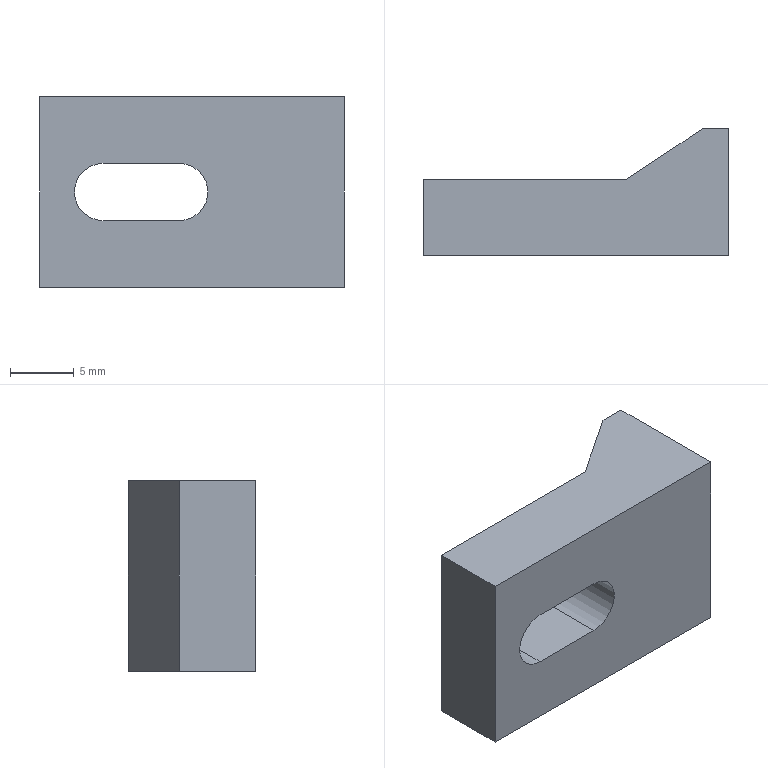Part | SolidWorks | features Extrusion 1, ICE 1 | 1 solid | 12 faces | box 24 x 10 x 15 mm | volume 2203 mm3 | plane 10 | cylinder 2 | commonest cylinder face diameters 4.5 x2
STEP:
#1=CARTESIAN_POINT('',(4.,1.,-7.5));
#2=VERTEX_POINT('',#1);
#3=CARTESIAN_POINT('',(10.,5.,-7.5));
#4=VERTEX_POINT('',#3);
#5=CARTESIAN_POINT('',(0.7692,-1.154,-7.5));
#6=DIRECTION('',(0.8321,0.5547,0.));
#7=VECTOR('',#6,1000.);
#8=LINE('',#5,#7);
#9=EDGE_CURVE('',#2,#4,#8,.T.);
#10=ORIENTED_EDGE('',*,*,#9,.F.);
#11=CARTESIAN_POINT('',(4.,1.,7.5));
#12=VERTEX_POINT('',#11);
#13=CARTESIAN_POINT('',(4.,1.,7.5));
#14=DIRECTION('',(0.,0.,-1.));
#15=VECTOR('',#14,1000.);
#16=LINE('',#13,#15);
#17=EDGE_CURVE('',#12,#2,#16,.T.);
#18=ORIENTED_EDGE('',*,*,#17,.F.);
#19=CARTESIAN_POINT('',(10.,5.,7.5));
#20=VERTEX_POINT('',#19);
#21=CARTESIAN_POINT('',(0.7692,-1.154,7.5));
#22=DIRECTION('',(0.8321,0.5547,0.));
#23=VECTOR('',#22,1000.);
#24=LINE('',#21,#23);
#25=EDGE_CURVE('',#12,#20,#24,.T.);
#26=ORIENTED_EDGE('',*,*,#25,.T.);
#27=CARTESIAN_POINT('',(10.,5.,7.5));
#28=DIRECTION('',(0.,0.,-1.));
#29=VECTOR('',#28,1000.);
#30=LINE('',#27,#29);
#31=EDGE_CURVE('',#20,#4,#30,.T.);
#32=ORIENTED_EDGE('',*,*,#31,.T.);
#33=EDGE_LOOP('',(#10,#18,#26,#32));
#34=FACE_OUTER_BOUND('',#33,.T.);
#35=CARTESIAN_POINT('',(0.7692,-1.154,7.5));
#36=DIRECTION('',(-0.5547,0.8321,0.));
#37=DIRECTION('',(-0.8321,-0.5547,0.));
#38=AXIS2_PLACEMENT_3D('',#35,#36,#37);
#39=PLANE('',#38);
#40=ADVANCED_FACE('',(#34),#39,.T.);
#41=CARTESIAN_POINT('',(-7.,1.,-2.25));
#42=VERTEX_POINT('',#41);
#43=CARTESIAN_POINT('',(-7.,1.,2.25));
#44=VERTEX_POINT('',#43);
#45=CARTESIAN_POINT('',(-7.,1.,0.));
#46=DIRECTION('',(0.,1.,0.));
#47=DIRECTION('',(0.,0.,1.));
#48=AXIS2_PLACEMENT_3D('',#45,#46,#47);
#49=CIRCLE('',#48,2.25);
#50=EDGE_CURVE('',#42,#44,#49,.T.);
#51=ORIENTED_EDGE('',*,*,#50,.F.);
#52=CARTESIAN_POINT('',(-1.,1.,-2.25));
#53=VERTEX_POINT('',#52);
#54=CARTESIAN_POINT('',(-7.,1.,-2.25));
#55=DIRECTION('',(-1.,0.,0.));
#56=VECTOR('',#55,1000.);
#57=LINE('',#54,#56);
#58=EDGE_CURVE('',#53,#42,#57,.T.);
#59=ORIENTED_EDGE('',*,*,#58,.F.);
#60=CARTESIAN_POINT('',(-1.,1.,2.25));
#61=VERTEX_POINT('',#60);
#62=CARTESIAN_POINT('',(-1.,1.,0.));
#63=DIRECTION('',(0.,1.,0.));
#64=DIRECTION('',(0.,0.,1.));
#65=AXIS2_PLACEMENT_3D('',#62,#63,#64);
#66=CIRCLE('',#65,2.25);
#67=EDGE_CURVE('',#61,#53,#66,.T.);
#68=ORIENTED_EDGE('',*,*,#67,.F.);
#69=CARTESIAN_POINT('',(-7.,1.,2.25));
#70=DIRECTION('',(1.,0.,0.));
#71=VECTOR('',#70,1000.);
#72=LINE('',#69,#71);
#73=EDGE_CURVE('',#44,#61,#72,.T.);
#74=ORIENTED_EDGE('',*,*,#73,.F.);
#75=EDGE_LOOP('',(#51,#59,#68,#74));
#76=FACE_BOUND('',#75,.T.);
#77=CARTESIAN_POINT('',(-12.,1.,-7.5));
#78=VERTEX_POINT('',#77);
#79=CARTESIAN_POINT('',(0.,1.,-7.5));
#80=DIRECTION('',(1.,0.,0.));
#81=VECTOR('',#80,1000.);
#82=LINE('',#79,#81);
#83=EDGE_CURVE('',#78,#2,#82,.T.);
#84=ORIENTED_EDGE('',*,*,#83,.F.);
#85=CARTESIAN_POINT('',(-12.,1.,7.5));
#86=VERTEX_POINT('',#85);
#87=CARTESIAN_POINT('',(-12.,1.,7.5));
#88=DIRECTION('',(0.,0.,-1.));
#89=VECTOR('',#88,1000.);
#90=LINE('',#87,#89);
#91=EDGE_CURVE('',#86,#78,#90,.T.);
#92=ORIENTED_EDGE('',*,*,#91,.F.);
#93=CARTESIAN_POINT('',(0.,1.,7.5));
#94=DIRECTION('',(1.,0.,0.));
#95=VECTOR('',#94,1000.);
#96=LINE('',#93,#95);
#97=EDGE_CURVE('',#86,#12,#96,.T.);
#98=ORIENTED_EDGE('',*,*,#97,.T.);
#99=ORIENTED_EDGE('',*,*,#17,.T.);
#100=EDGE_LOOP('',(#84,#92,#98,#99));
#101=FACE_OUTER_BOUND('',#100,.T.);
#102=CARTESIAN_POINT('',(0.,1.,7.5));
#103=DIRECTION('',(0.,1.,0.));
#104=DIRECTION('',(-1.,0.,0.));
#105=AXIS2_PLACEMENT_3D('',#102,#103,#104);
#106=PLANE('',#105);
#107=ADVANCED_FACE('',(#76,#101),#106,.T.);
#108=CARTESIAN_POINT('',(-12.,-5.,-7.5));
#109=VERTEX_POINT('',#108);
#110=CARTESIAN_POINT('',(-12.,0.,-7.5));
#111=DIRECTION('',(0.,1.,0.));
#112=VECTOR('',#111,1000.);
#113=LINE('',#110,#112);
#114=EDGE_CURVE('',#109,#78,#113,.T.);
#115=ORIENTED_EDGE('',*,*,#114,.F.);
#116=CARTESIAN_POINT('',(-12.,-5.,7.5));
#117=VERTEX_POINT('',#116);
#118=CARTESIAN_POINT('',(-12.,-5.,7.5));
#119=DIRECTION('',(0.,0.,-1.));
#120=VECTOR('',#119,1000.);
#121=LINE('',#118,#120);
#122=EDGE_CURVE('',#117,#109,#121,.T.);
#123=ORIENTED_EDGE('',*,*,#122,.F.);
#124=CARTESIAN_POINT('',(-12.,0.,7.5));
#125=DIRECTION('',(0.,1.,0.));
#126=VECTOR('',#125,1000.);
#127=LINE('',#124,#126);
#128=EDGE_CURVE('',#117,#86,#127,.T.);
#129=ORIENTED_EDGE('',*,*,#128,.T.);
#130=ORIENTED_EDGE('',*,*,#91,.T.);
#131=EDGE_LOOP('',(#115,#123,#129,#130));
#132=FACE_OUTER_BOUND('',#131,.T.);
#133=CARTESIAN_POINT('',(-12.,0.,7.5));
#134=DIRECTION('',(-1.,0.,0.));
#135=DIRECTION('',(0.,0.,1.));
#136=AXIS2_PLACEMENT_3D('',#133,#134,#135);
#137=PLANE('',#136);
#138=ADVANCED_FACE('',(#132),#137,.T.);
#139=CARTESIAN_POINT('',(-7.,-5.,-2.25));
#140=VERTEX_POINT('',#139);
#141=CARTESIAN_POINT('',(-1.,-5.,-2.25));
#142=VERTEX_POINT('',#141);
#143=CARTESIAN_POINT('',(-7.,-5.,-2.25));
#144=DIRECTION('',(1.,0.,0.));
#145=VECTOR('',#144,1000.);
#146=LINE('',#143,#145);
#147=EDGE_CURVE('',#140,#142,#146,.T.);
#148=ORIENTED_EDGE('',*,*,#147,.F.);
#149=CARTESIAN_POINT('',(-7.,-5.,2.25));
#150=VERTEX_POINT('',#149);
#151=CARTESIAN_POINT('',(-7.,-5.,0.));
#152=DIRECTION('',(0.,-1.,0.));
#153=DIRECTION('',(0.,0.,1.));
#154=AXIS2_PLACEMENT_3D('',#151,#152,#153);
#155=CIRCLE('',#154,2.25);
#156=EDGE_CURVE('',#150,#140,#155,.T.);
#157=ORIENTED_EDGE('',*,*,#156,.F.);
#158=CARTESIAN_POINT('',(-1.,-5.,2.25));
#159=VERTEX_POINT('',#158);
#160=CARTESIAN_POINT('',(-7.,-5.,2.25));
#161=DIRECTION('',(-1.,0.,0.));
#162=VECTOR('',#161,1000.);
#163=LINE('',#160,#162);
#164=EDGE_CURVE('',#159,#150,#163,.T.);
#165=ORIENTED_EDGE('',*,*,#164,.F.);
#166=CARTESIAN_POINT('',(-1.,-5.,0.));
#167=DIRECTION('',(0.,-1.,0.));
#168=DIRECTION('',(0.,0.,1.));
#169=AXIS2_PLACEMENT_3D('',#166,#167,#168);
#170=CIRCLE('',#169,2.25);
#171=EDGE_CURVE('',#142,#159,#170,.T.);
#172=ORIENTED_EDGE('',*,*,#171,.F.);
#173=EDGE_LOOP('',(#148,#157,#165,#172));
#174=FACE_BOUND('',#173,.T.);
#175=CARTESIAN_POINT('',(12.,-5.,-7.5));
#176=VERTEX_POINT('',#175);
#177=CARTESIAN_POINT('',(0.,-5.,-7.5));
#178=DIRECTION('',(1.,0.,0.));
#179=VECTOR('',#178,1000.);
#180=LINE('',#177,#179);
#181=EDGE_CURVE('',#109,#176,#180,.T.);
#182=ORIENTED_EDGE('',*,*,#181,.T.);
#183=CARTESIAN_POINT('',(12.,-5.,7.5));
#184=VERTEX_POINT('',#183);
#185=CARTESIAN_POINT('',(12.,-5.,7.5));
#186=DIRECTION('',(0.,0.,-1.));
#187=VECTOR('',#186,1000.);
#188=LINE('',#185,#187);
#189=EDGE_CURVE('',#184,#176,#188,.T.);
#190=ORIENTED_EDGE('',*,*,#189,.F.);
#191=CARTESIAN_POINT('',(0.,-5.,7.5));
#192=DIRECTION('',(1.,0.,0.));
#193=VECTOR('',#192,1000.);
#194=LINE('',#191,#193);
#195=EDGE_CURVE('',#117,#184,#194,.T.);
#196=ORIENTED_EDGE('',*,*,#195,.F.);
#197=ORIENTED_EDGE('',*,*,#122,.T.);
#198=EDGE_LOOP('',(#182,#190,#196,#197));
#199=FACE_OUTER_BOUND('',#198,.T.);
#200=CARTESIAN_POINT('',(0.,-5.,7.5));
#201=DIRECTION('',(0.,1.,0.));
#202=DIRECTION('',(0.,0.,1.));
#203=AXIS2_PLACEMENT_3D('',#200,#201,#202);
#204=PLANE('',#203);
#205=ADVANCED_FACE('',(#174,#199),#204,.F.);
#206=CARTESIAN_POINT('',(12.,5.,-7.5));
#207=VERTEX_POINT('',#206);
#208=CARTESIAN_POINT('',(12.,0.,-7.5));
#209=DIRECTION('',(0.,1.,0.));
#210=VECTOR('',#209,1000.);
#211=LINE('',#208,#210);
#212=EDGE_CURVE('',#176,#207,#211,.T.);
#213=ORIENTED_EDGE('',*,*,#212,.T.);
#214=CARTESIAN_POINT('',(12.,5.,7.5));
#215=VERTEX_POINT('',#214);
#216=CARTESIAN_POINT('',(12.,5.,7.5));
#217=DIRECTION('',(0.,0.,-1.));
#218=VECTOR('',#217,1000.);
#219=LINE('',#216,#218);
#220=EDGE_CURVE('',#215,#207,#219,.T.);
#221=ORIENTED_EDGE('',*,*,#220,.F.);
#222=CARTESIAN_POINT('',(12.,0.,7.5));
#223=DIRECTION('',(0.,1.,0.));
#224=VECTOR('',#223,1000.);
#225=LINE('',#222,#224);
#226=EDGE_CURVE('',#184,#215,#225,.T.);
#227=ORIENTED_EDGE('',*,*,#226,.F.);
#228=ORIENTED_EDGE('',*,*,#189,.T.);
#229=EDGE_LOOP('',(#213,#221,#227,#228));
#230=FACE_OUTER_BOUND('',#229,.T.);
#231=CARTESIAN_POINT('',(12.,0.,7.5));
#232=DIRECTION('',(-1.,0.,0.));
#233=DIRECTION('',(0.,0.,1.));
#234=AXIS2_PLACEMENT_3D('',#231,#232,#233);
#235=PLANE('',#234);
#236=ADVANCED_FACE('',(#230),#235,.F.);
#237=CARTESIAN_POINT('',(0.,5.,-7.5));
#238=DIRECTION('',(1.,0.,0.));
#239=VECTOR('',#238,1000.);
#240=LINE('',#237,#239);
#241=EDGE_CURVE('',#4,#207,#240,.T.);
#242=ORIENTED_EDGE('',*,*,#241,.F.);
#243=ORIENTED_EDGE('',*,*,#31,.F.);
#244=CARTESIAN_POINT('',(0.,5.,7.5));
#245=DIRECTION('',(1.,0.,0.));
#246=VECTOR('',#245,1000.);
#247=LINE('',#244,#246);
#248=EDGE_CURVE('',#20,#215,#247,.T.);
#249=ORIENTED_EDGE('',*,*,#248,.T.);
#250=ORIENTED_EDGE('',*,*,#220,.T.);
#251=EDGE_LOOP('',(#242,#243,#249,#250));
#252=FACE_OUTER_BOUND('',#251,.T.);
#253=CARTESIAN_POINT('',(0.,5.,7.5));
#254=DIRECTION('',(0.,1.,0.));
#255=DIRECTION('',(0.,0.,1.));
#256=AXIS2_PLACEMENT_3D('',#253,#254,#255);
#257=PLANE('',#256);
#258=ADVANCED_FACE('',(#252),#257,.T.);
#259=ORIENTED_EDGE('',*,*,#25,.F.);
#260=ORIENTED_EDGE('',*,*,#97,.F.);
#261=ORIENTED_EDGE('',*,*,#128,.F.);
#262=ORIENTED_EDGE('',*,*,#195,.T.);
#263=ORIENTED_EDGE('',*,*,#226,.T.);
#264=ORIENTED_EDGE('',*,*,#248,.F.);
#265=EDGE_LOOP('',(#259,#260,#261,#262,#263,#264));
#266=FACE_OUTER_BOUND('',#265,.T.);
#267=CARTESIAN_POINT('',(0.,0.,7.5));
#268=DIRECTION('',(0.,0.,1.));
#269=DIRECTION('',(1.,0.,0.));
#270=AXIS2_PLACEMENT_3D('',#267,#268,#269);
#271=PLANE('',#270);
#272=ADVANCED_FACE('',(#266),#271,.T.);
#273=ORIENTED_EDGE('',*,*,#9,.T.);
#274=ORIENTED_EDGE('',*,*,#241,.T.);
#275=ORIENTED_EDGE('',*,*,#212,.F.);
#276=ORIENTED_EDGE('',*,*,#181,.F.);
#277=ORIENTED_EDGE('',*,*,#114,.T.);
#278=ORIENTED_EDGE('',*,*,#83,.T.);
#279=EDGE_LOOP('',(#273,#274,#275,#276,#277,#278));
#280=FACE_OUTER_BOUND('',#279,.T.);
#281=CARTESIAN_POINT('',(0.,0.,-7.5));
#282=DIRECTION('',(0.,0.,1.));
#283=DIRECTION('',(1.,0.,0.));
#284=AXIS2_PLACEMENT_3D('',#281,#282,#283);
#285=PLANE('',#284);
#286=ADVANCED_FACE('',(#280),#285,.F.);
#287=ORIENTED_EDGE('',*,*,#156,.T.);
#288=CARTESIAN_POINT('',(-7.,-5.001,-2.25));
#289=DIRECTION('',(0.,1.,0.));
#290=VECTOR('',#289,1000.);
#291=LINE('',#288,#290);
#292=EDGE_CURVE('',#140,#42,#291,.T.);
#293=ORIENTED_EDGE('',*,*,#292,.T.);
#294=ORIENTED_EDGE('',*,*,#50,.T.);
#295=CARTESIAN_POINT('',(-7.,-5.001,2.25));
#296=DIRECTION('',(0.,1.,0.));
#297=VECTOR('',#296,1000.);
#298=LINE('',#295,#297);
#299=EDGE_CURVE('',#150,#44,#298,.T.);
#300=ORIENTED_EDGE('',*,*,#299,.F.);
#301=EDGE_LOOP('',(#287,#293,#294,#300));
#302=FACE_OUTER_BOUND('',#301,.T.);
#303=CARTESIAN_POINT('',(-7.,-5.001,0.));
#304=DIRECTION('',(0.,1.,0.));
#305=DIRECTION('',(0.,0.,1.));
#306=AXIS2_PLACEMENT_3D('',#303,#304,#305);
#307=CYLINDRICAL_SURFACE('',#306,2.25);
#308=ADVANCED_FACE('',(#302),#307,.F.);
#309=ORIENTED_EDGE('',*,*,#147,.T.);
#310=CARTESIAN_POINT('',(-1.,-5.001,-2.25));
#311=DIRECTION('',(0.,1.,0.));
#312=VECTOR('',#311,1000.);
#313=LINE('',#310,#312);
#314=EDGE_CURVE('',#142,#53,#313,.T.);
#315=ORIENTED_EDGE('',*,*,#314,.T.);
#316=ORIENTED_EDGE('',*,*,#58,.T.);
#317=ORIENTED_EDGE('',*,*,#292,.F.);
#318=EDGE_LOOP('',(#309,#315,#316,#317));
#319=FACE_OUTER_BOUND('',#318,.T.);
#320=CARTESIAN_POINT('',(-7.,-5.001,-2.25));
#321=DIRECTION('',(0.,0.,-1.));
#322=DIRECTION('',(-1.,0.,0.));
#323=AXIS2_PLACEMENT_3D('',#320,#321,#322);
#324=PLANE('',#323);
#325=ADVANCED_FACE('',(#319),#324,.F.);
#326=ORIENTED_EDGE('',*,*,#171,.T.);
#327=CARTESIAN_POINT('',(-1.,-5.001,2.25));
#328=DIRECTION('',(0.,1.,0.));
#329=VECTOR('',#328,1000.);
#330=LINE('',#327,#329);
#331=EDGE_CURVE('',#159,#61,#330,.T.);
#332=ORIENTED_EDGE('',*,*,#331,.T.);
#333=ORIENTED_EDGE('',*,*,#67,.T.);
#334=ORIENTED_EDGE('',*,*,#314,.F.);
#335=EDGE_LOOP('',(#326,#332,#333,#334));
#336=FACE_OUTER_BOUND('',#335,.T.);
#337=CARTESIAN_POINT('',(-1.,-5.001,0.));
#338=DIRECTION('',(0.,1.,0.));
#339=DIRECTION('',(0.,0.,1.));
#340=AXIS2_PLACEMENT_3D('',#337,#338,#339);
#341=CYLINDRICAL_SURFACE('',#340,2.25);
#342=ADVANCED_FACE('',(#336),#341,.F.);
#343=ORIENTED_EDGE('',*,*,#164,.T.);
#344=ORIENTED_EDGE('',*,*,#299,.T.);
#345=ORIENTED_EDGE('',*,*,#73,.T.);
#346=ORIENTED_EDGE('',*,*,#331,.F.);
#347=EDGE_LOOP('',(#343,#344,#345,#346));
#348=FACE_OUTER_BOUND('',#347,.T.);
#349=CARTESIAN_POINT('',(-7.,-5.001,2.25));
#350=DIRECTION('',(0.,0.,1.));
#351=DIRECTION('',(1.,0.,0.));
#352=AXIS2_PLACEMENT_3D('',#349,#350,#351);
#353=PLANE('',#352);
#354=ADVANCED_FACE('',(#348),#353,.F.);
#355=CLOSED_SHELL('',(#40,#107,#138,#205,#236,#258,#272,#286,#308,#325,#342,#354));
#356=MANIFOLD_SOLID_BREP('',#355);
#357=CARTESIAN_POINT('',(0.,0.,0.));
#358=DIRECTION('',(0.,0.,1.));
#359=DIRECTION('',(1.,0.,0.));
#360=AXIS2_PLACEMENT_3D('',#357,#358,#359);
#361=(LENGTH_UNIT()NAMED_UNIT(*)SI_UNIT(.MILLI.,.METRE.));
#362=UNCERTAINTY_MEASURE_WITH_UNIT(LENGTH_MEASURE(0.00001),#361,'','');
#363=(NAMED_UNIT(*)PLANE_ANGLE_UNIT()SI_UNIT($,.RADIAN.));
#364=(NAMED_UNIT(*)SI_UNIT($,.STERADIAN.)SOLID_ANGLE_UNIT());
#365=(GEOMETRIC_REPRESENTATION_CONTEXT(3)GLOBAL_UNCERTAINTY_ASSIGNED_CONTEXT((#362))GLOBAL_UNIT_ASSIGNED_CONTEXT((#361,#363,#364))REPRESENTATION_CONTEXT('',''));
#366=ADVANCED_BREP_SHAPE_REPRESENTATION('',(#356,#360),#365);